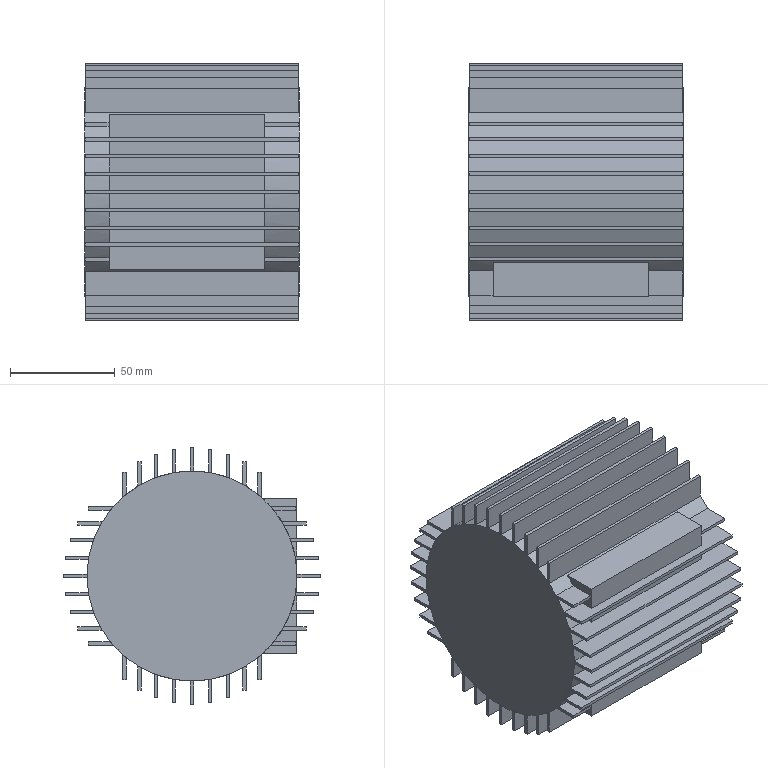Part | STEP file | PRODUCT_NAME_39_default | 1 solid | 216 faces | box 102 x 122 x 122 mm | volume 884304 mm3 | plane 214 | cylinder 2 | commonest cylinder face diameters 100 x2